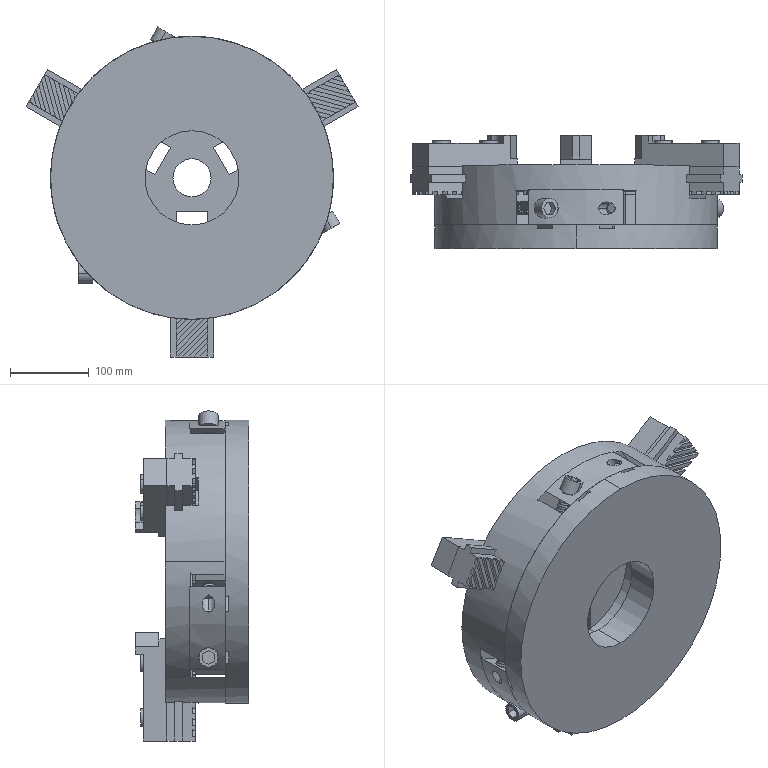Part | SolidWorks | features ReferencePattern 12, LocalCirPattern 4, CompositeCurve 3, Cut 1 | 23 solids | 1236 faces | box 422.408 x 144 x 419.924 mm | volume 8918159 mm3 | plane 799 | cylinder 425 | spline 12 | commonest cylinder face diameters 12 x255 15 x36 180 x31 200 x30 16 x18 25 x15